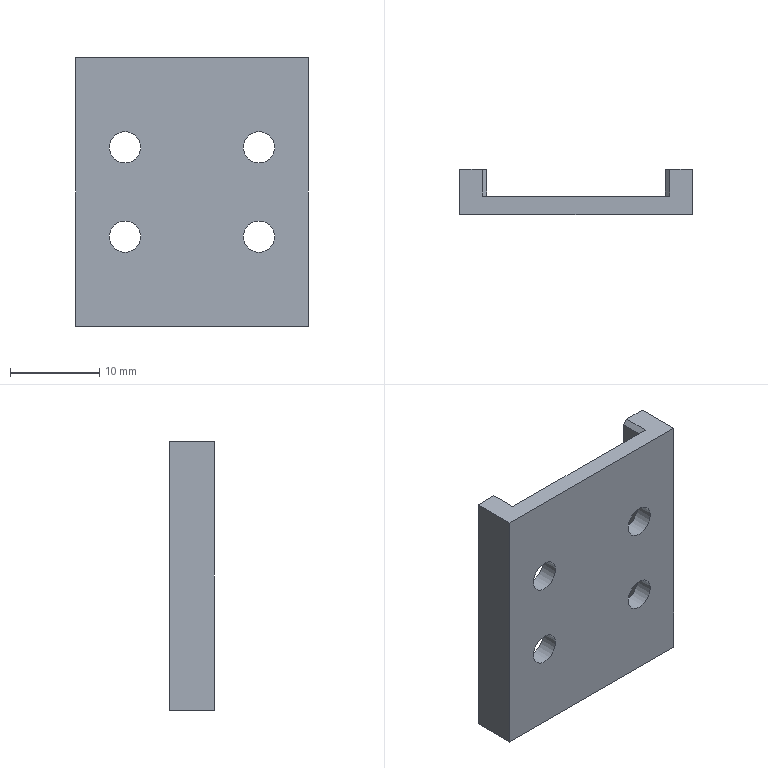CAM job | NX | 3+2 milling, drilling | part box 26 x 5 x 30 mm | stock box 26 x 5 x 31 mm
Tools:
number,name,description,diameter,corner_radius,flute_length,length,flutes
1,D50,Milling Tool-5 Parameters,50.0,0.0,50.0,75.0,2
10,D10,Milling Tool-5 Parameters,10.0,0.0,50.0,75.0,2
6,D6JING,Milling Tool-5 Parameters,6.0,0.0,50.0,75.0,2
2,ZXZ,Milling Tool-5 Parameters,6.0,0.0,50.0,75.0,2
13,3.5ZT,Drilling Tool,3.5,0.0,35.0,50.0,2
7,D4A45,Milling Tool-5 Parameters,4.0,0.0,50.0,75.0,2
Operations:
program,operation,operation_type,tool,method,geometry_group,spindle_rpm,surface_speed,feed_per_tooth,feed_cut,feed_plunge,cut_length_mm,path_length_mm,cut_time_min,machine_time_min
1,FLOOR_WALL,VolumeBased25DMillingOperation,D50,METHOD,A,2000.0,314.0,0.2,800.0,100.0,92.0,146.0,0.115,0.1204
1,DRILLING,Operation,ZXZ,METHOD,A,3500.0,65.0,0.0357,250.0,0.0,16.0,137.178,0.064,0.0761
1,DRILLING_COPY,Operation,3.5ZT,METHOD,A,2000.0,21.0,0.0375,150.0,0.0,42.206,189.59,0.2814,0.2961
1,FLOOR_WALL_1,VolumeBased25DMillingOperation,D10,METHOD,A,3000.0,94.0,0.3333,2000.0,1000.0,3082.062,3232.597,1.567,1.582
1,FLOOR_WALL_1_COPY,VolumeBased25DMillingOperation,D6JING,METHOD,A,6000.0,113.0,0.0833,1000.0,1000.0,322.642,409.408,0.3226,0.3319
1,PLANAR_MILL,PlanarMilling,D4A45,METHOD,A,7500.0,141.0,0.0833,1250.0,100.0,150.581,297.581,0.1205,0.1352
1,PLANAR_MILL_COPY,PlanarMilling,D4A45,METHOD,A,7500.0,141.0,0.0833,1250.0,100.0,42.147,205.799,0.0337,0.0501
1,DRILLING_COPY_1,Operation,D4A45,METHOD,A,3500.0,65.0,0.0357,250.0,0.0,19.6,150.348,0.0784,0.0915
1,刀补,VolumeBased25DMillingOperation,D6JING,METHOD,A,6000.0,113.0,0.0833,1000.0,1000.0,86.465,168.683,0.0865,0.0951